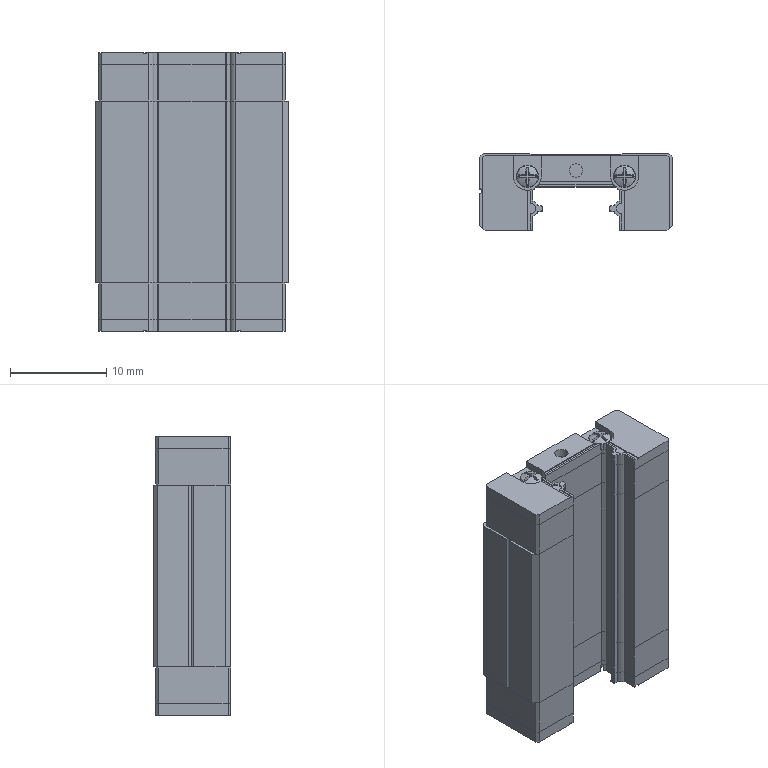Part | STEP file | 5 solids | 532 faces | box 20 x 8 x 28.991 mm | volume 3251 mm3 | plane 331 | spline 93 | cylinder 84 | torus 8 | sphere 8 | cone 8 | commonest cylinder face diameters 0.18 x20 1.616 x20 2.328 x8 2.4 x8 2.91 x8 3 x8